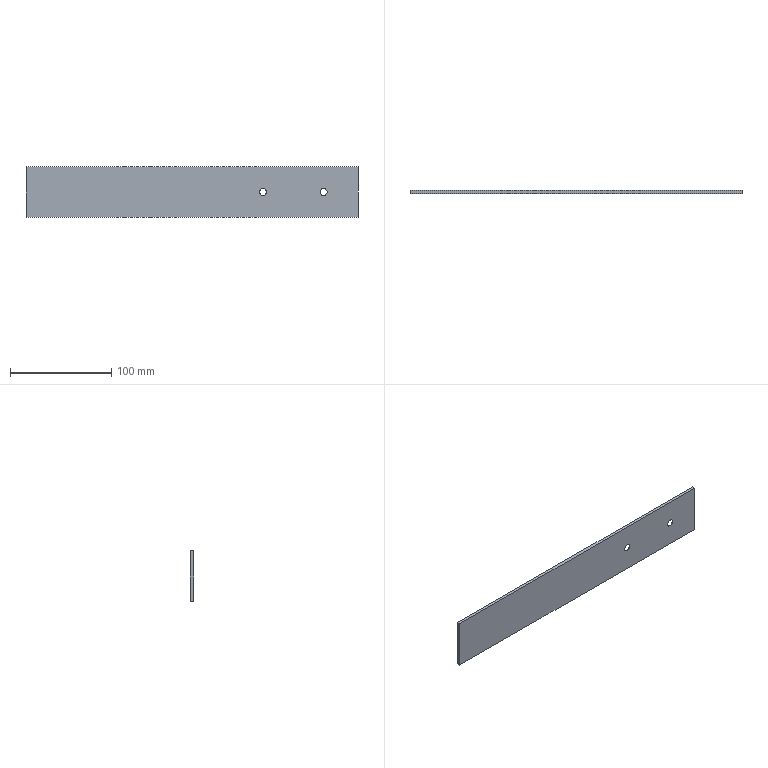Part | STEP file | Guard plate | 1 solid | 10 faces | box 328 x 3 x 50 mm | volume 48733 mm3 | plane 6 | cone 4
STEP:
#1=CARTESIAN_POINT('',(30.,-3.,3.4));
#2=VERTEX_POINT('',#1);
#3=CARTESIAN_POINT('',(30.,-3.,-3.4));
#4=VERTEX_POINT('',#3);
#5=CARTESIAN_POINT('',(30.,-3.,0.));
#6=DIRECTION('',(0.,-1.,0.));
#7=DIRECTION('',(0.,0.,1.));
#8=AXIS2_PLACEMENT_3D('',#5,#6,#7);
#9=CIRCLE('',#8,3.4);
#10=EDGE_CURVE('',#2,#4,#9,.T.);
#11=ORIENTED_EDGE('',*,*,#10,.T.);
#12=CARTESIAN_POINT('',(30.,0.,-6.4));
#13=VERTEX_POINT('',#12);
#14=CARTESIAN_POINT('',(30.,0.,-6.4));
#15=DIRECTION('',(0.,0.7071,-0.7071));
#16=VECTOR('',#15,1000.);
#17=LINE('',#14,#16);
#18=EDGE_CURVE('',#4,#13,#17,.T.);
#19=ORIENTED_EDGE('',*,*,#18,.T.);
#20=CARTESIAN_POINT('',(30.,0.,6.4));
#21=VERTEX_POINT('',#20);
#22=CARTESIAN_POINT('',(30.,0.,0.));
#23=DIRECTION('',(0.,-1.,0.));
#24=DIRECTION('',(0.,0.,1.));
#25=AXIS2_PLACEMENT_3D('',#22,#23,#24);
#26=CIRCLE('',#25,6.4);
#27=EDGE_CURVE('',#21,#13,#26,.T.);
#28=ORIENTED_EDGE('',*,*,#27,.F.);
#29=CARTESIAN_POINT('',(30.,0.,6.4));
#30=DIRECTION('',(0.,0.7071,0.7071));
#31=VECTOR('',#30,1000.);
#32=LINE('',#29,#31);
#33=EDGE_CURVE('',#2,#21,#32,.T.);
#34=ORIENTED_EDGE('',*,*,#33,.F.);
#35=EDGE_LOOP('',(#11,#19,#28,#34));
#36=FACE_OUTER_BOUND('',#35,.T.);
#37=CARTESIAN_POINT('',(30.,0.,0.));
#38=DIRECTION('',(0.,1.,0.));
#39=DIRECTION('',(0.,0.,1.));
#40=AXIS2_PLACEMENT_3D('',#37,#38,#39);
#41=CONICAL_SURFACE('',#40,6.4,0.7854);
#42=ADVANCED_FACE('',(#36),#41,.F.);
#43=CARTESIAN_POINT('',(-30.,-3.,3.4));
#44=VERTEX_POINT('',#43);
#45=CARTESIAN_POINT('',(-30.,-3.,-3.4));
#46=VERTEX_POINT('',#45);
#47=CARTESIAN_POINT('',(-30.,-3.,0.));
#48=DIRECTION('',(0.,-1.,0.));
#49=DIRECTION('',(0.,0.,1.));
#50=AXIS2_PLACEMENT_3D('',#47,#48,#49);
#51=CIRCLE('',#50,3.4);
#52=EDGE_CURVE('',#44,#46,#51,.T.);
#53=ORIENTED_EDGE('',*,*,#52,.T.);
#54=CARTESIAN_POINT('',(-30.,0.,-6.4));
#55=VERTEX_POINT('',#54);
#56=CARTESIAN_POINT('',(-30.,0.,-6.4));
#57=DIRECTION('',(0.,0.7071,-0.7071));
#58=VECTOR('',#57,1000.);
#59=LINE('',#56,#58);
#60=EDGE_CURVE('',#46,#55,#59,.T.);
#61=ORIENTED_EDGE('',*,*,#60,.T.);
#62=CARTESIAN_POINT('',(-30.,0.,6.4));
#63=VERTEX_POINT('',#62);
#64=CARTESIAN_POINT('',(-30.,0.,0.));
#65=DIRECTION('',(0.,-1.,0.));
#66=DIRECTION('',(0.,0.,1.));
#67=AXIS2_PLACEMENT_3D('',#64,#65,#66);
#68=CIRCLE('',#67,6.4);
#69=EDGE_CURVE('',#63,#55,#68,.T.);
#70=ORIENTED_EDGE('',*,*,#69,.F.);
#71=CARTESIAN_POINT('',(-30.,0.,6.4));
#72=DIRECTION('',(0.,0.7071,0.7071));
#73=VECTOR('',#72,1000.);
#74=LINE('',#71,#73);
#75=EDGE_CURVE('',#44,#63,#74,.T.);
#76=ORIENTED_EDGE('',*,*,#75,.F.);
#77=EDGE_LOOP('',(#53,#61,#70,#76));
#78=FACE_OUTER_BOUND('',#77,.T.);
#79=CARTESIAN_POINT('',(-30.,0.,0.));
#80=DIRECTION('',(0.,1.,0.));
#81=DIRECTION('',(0.,0.,1.));
#82=AXIS2_PLACEMENT_3D('',#79,#80,#81);
#83=CONICAL_SURFACE('',#82,6.4,0.7854);
#84=ADVANCED_FACE('',(#78),#83,.F.);
#85=CARTESIAN_POINT('',(-264.,-3.,25.));
#86=VERTEX_POINT('',#85);
#87=CARTESIAN_POINT('',(64.,-3.,25.));
#88=VERTEX_POINT('',#87);
#89=CARTESIAN_POINT('',(0.,-3.,25.));
#90=DIRECTION('',(1.,0.,0.));
#91=VECTOR('',#90,1000.);
#92=LINE('',#89,#91);
#93=EDGE_CURVE('',#86,#88,#92,.T.);
#94=ORIENTED_EDGE('',*,*,#93,.F.);
#95=CARTESIAN_POINT('',(-264.,-3.,-25.));
#96=VERTEX_POINT('',#95);
#97=CARTESIAN_POINT('',(-264.,-3.,-25.));
#98=DIRECTION('',(0.,0.,1.));
#99=VECTOR('',#98,1000.);
#100=LINE('',#97,#99);
#101=EDGE_CURVE('',#96,#86,#100,.T.);
#102=ORIENTED_EDGE('',*,*,#101,.F.);
#103=CARTESIAN_POINT('',(64.,-3.,-25.));
#104=VERTEX_POINT('',#103);
#105=CARTESIAN_POINT('',(0.,-3.,-25.));
#106=DIRECTION('',(-1.,0.,0.));
#107=VECTOR('',#106,1000.);
#108=LINE('',#105,#107);
#109=EDGE_CURVE('',#104,#96,#108,.T.);
#110=ORIENTED_EDGE('',*,*,#109,.F.);
#111=CARTESIAN_POINT('',(64.,-3.,0.));
#112=DIRECTION('',(0.,0.,-1.));
#113=VECTOR('',#112,1000.);
#114=LINE('',#111,#113);
#115=EDGE_CURVE('',#88,#104,#114,.T.);
#116=ORIENTED_EDGE('',*,*,#115,.F.);
#117=EDGE_LOOP('',(#94,#102,#110,#116));
#118=FACE_OUTER_BOUND('',#117,.T.);
#119=ORIENTED_EDGE('',*,*,#10,.F.);
#120=CARTESIAN_POINT('',(30.,-3.,0.));
#121=DIRECTION('',(0.,-1.,0.));
#122=DIRECTION('',(0.,0.,1.));
#123=AXIS2_PLACEMENT_3D('',#120,#121,#122);
#124=CIRCLE('',#123,3.4);
#125=EDGE_CURVE('',#4,#2,#124,.T.);
#126=ORIENTED_EDGE('',*,*,#125,.F.);
#127=EDGE_LOOP('',(#119,#126));
#128=FACE_BOUND('',#127,.T.);
#129=ORIENTED_EDGE('',*,*,#52,.F.);
#130=CARTESIAN_POINT('',(-30.,-3.,0.));
#131=DIRECTION('',(0.,-1.,0.));
#132=DIRECTION('',(0.,0.,1.));
#133=AXIS2_PLACEMENT_3D('',#130,#131,#132);
#134=CIRCLE('',#133,3.4);
#135=EDGE_CURVE('',#46,#44,#134,.T.);
#136=ORIENTED_EDGE('',*,*,#135,.F.);
#137=EDGE_LOOP('',(#129,#136));
#138=FACE_BOUND('',#137,.T.);
#139=CARTESIAN_POINT('',(0.,-3.,0.));
#140=DIRECTION('',(0.,1.,0.));
#141=DIRECTION('',(0.,0.,1.));
#142=AXIS2_PLACEMENT_3D('',#139,#140,#141);
#143=PLANE('',#142);
#144=ADVANCED_FACE('',(#118,#128,#138),#143,.F.);
#145=ORIENTED_EDGE('',*,*,#115,.T.);
#146=CARTESIAN_POINT('',(64.,0.,-25.));
#147=VERTEX_POINT('',#146);
#148=CARTESIAN_POINT('',(64.,-3.,-25.));
#149=DIRECTION('',(0.,1.,0.));
#150=VECTOR('',#149,1000.);
#151=LINE('',#148,#150);
#152=EDGE_CURVE('',#104,#147,#151,.T.);
#153=ORIENTED_EDGE('',*,*,#152,.T.);
#154=CARTESIAN_POINT('',(64.,0.,25.));
#155=VERTEX_POINT('',#154);
#156=CARTESIAN_POINT('',(64.,0.,-25.));
#157=DIRECTION('',(0.,0.,1.));
#158=VECTOR('',#157,1000.);
#159=LINE('',#156,#158);
#160=EDGE_CURVE('',#147,#155,#159,.T.);
#161=ORIENTED_EDGE('',*,*,#160,.T.);
#162=CARTESIAN_POINT('',(64.,-3.,25.));
#163=DIRECTION('',(0.,-1.,0.));
#164=VECTOR('',#163,1000.);
#165=LINE('',#162,#164);
#166=EDGE_CURVE('',#155,#88,#165,.T.);
#167=ORIENTED_EDGE('',*,*,#166,.T.);
#168=EDGE_LOOP('',(#145,#153,#161,#167));
#169=FACE_OUTER_BOUND('',#168,.T.);
#170=CARTESIAN_POINT('',(64.,-3.,-25.));
#171=DIRECTION('',(1.,0.,0.));
#172=DIRECTION('',(0.,0.,-1.));
#173=AXIS2_PLACEMENT_3D('',#170,#171,#172);
#174=PLANE('',#173);
#175=ADVANCED_FACE('',(#169),#174,.T.);
#176=ORIENTED_EDGE('',*,*,#93,.T.);
#177=ORIENTED_EDGE('',*,*,#166,.F.);
#178=CARTESIAN_POINT('',(-264.,0.,25.));
#179=VERTEX_POINT('',#178);
#180=CARTESIAN_POINT('',(-64.,0.,25.));
#181=DIRECTION('',(-1.,0.,0.));
#182=VECTOR('',#181,1000.);
#183=LINE('',#180,#182);
#184=EDGE_CURVE('',#155,#179,#183,.T.);
#185=ORIENTED_EDGE('',*,*,#184,.T.);
#186=CARTESIAN_POINT('',(-264.,-3.,25.));
#187=DIRECTION('',(0.,1.,0.));
#188=VECTOR('',#187,1000.);
#189=LINE('',#186,#188);
#190=EDGE_CURVE('',#86,#179,#189,.T.);
#191=ORIENTED_EDGE('',*,*,#190,.F.);
#192=EDGE_LOOP('',(#176,#177,#185,#191));
#193=FACE_OUTER_BOUND('',#192,.T.);
#194=CARTESIAN_POINT('',(-64.,-3.,25.));
#195=DIRECTION('',(0.,0.,1.));
#196=DIRECTION('',(1.,0.,0.));
#197=AXIS2_PLACEMENT_3D('',#194,#195,#196);
#198=PLANE('',#197);
#199=ADVANCED_FACE('',(#193),#198,.T.);
#200=ORIENTED_EDGE('',*,*,#109,.T.);
#201=CARTESIAN_POINT('',(-264.,0.,-25.));
#202=VERTEX_POINT('',#201);
#203=CARTESIAN_POINT('',(-264.,0.,-25.));
#204=DIRECTION('',(0.,-1.,0.));
#205=VECTOR('',#204,1000.);
#206=LINE('',#203,#205);
#207=EDGE_CURVE('',#202,#96,#206,.T.);
#208=ORIENTED_EDGE('',*,*,#207,.F.);
#209=CARTESIAN_POINT('',(-64.,0.,-25.));
#210=DIRECTION('',(1.,0.,0.));
#211=VECTOR('',#210,1000.);
#212=LINE('',#209,#211);
#213=EDGE_CURVE('',#202,#147,#212,.T.);
#214=ORIENTED_EDGE('',*,*,#213,.T.);
#215=ORIENTED_EDGE('',*,*,#152,.F.);
#216=EDGE_LOOP('',(#200,#208,#214,#215));
#217=FACE_OUTER_BOUND('',#216,.T.);
#218=CARTESIAN_POINT('',(-64.,-3.,-25.));
#219=DIRECTION('',(0.,0.,-1.));
#220=DIRECTION('',(-1.,0.,0.));
#221=AXIS2_PLACEMENT_3D('',#218,#219,#220);
#222=PLANE('',#221);
#223=ADVANCED_FACE('',(#217),#222,.T.);
#224=ORIENTED_EDGE('',*,*,#18,.F.);
#225=ORIENTED_EDGE('',*,*,#125,.T.);
#226=ORIENTED_EDGE('',*,*,#33,.T.);
#227=CARTESIAN_POINT('',(30.,0.,0.));
#228=DIRECTION('',(0.,-1.,0.));
#229=DIRECTION('',(0.,0.,1.));
#230=AXIS2_PLACEMENT_3D('',#227,#228,#229);
#231=CIRCLE('',#230,6.4);
#232=EDGE_CURVE('',#13,#21,#231,.T.);
#233=ORIENTED_EDGE('',*,*,#232,.F.);
#234=EDGE_LOOP('',(#224,#225,#226,#233));
#235=FACE_OUTER_BOUND('',#234,.T.);
#236=CARTESIAN_POINT('',(30.,0.,0.));
#237=DIRECTION('',(0.,1.,0.));
#238=DIRECTION('',(0.,0.,1.));
#239=AXIS2_PLACEMENT_3D('',#236,#237,#238);
#240=CONICAL_SURFACE('',#239,6.4,0.7854);
#241=ADVANCED_FACE('',(#235),#240,.F.);
#242=ORIENTED_EDGE('',*,*,#60,.F.);
#243=ORIENTED_EDGE('',*,*,#135,.T.);
#244=ORIENTED_EDGE('',*,*,#75,.T.);
#245=CARTESIAN_POINT('',(-30.,0.,0.));
#246=DIRECTION('',(0.,-1.,0.));
#247=DIRECTION('',(0.,0.,1.));
#248=AXIS2_PLACEMENT_3D('',#245,#246,#247);
#249=CIRCLE('',#248,6.4);
#250=EDGE_CURVE('',#55,#63,#249,.T.);
#251=ORIENTED_EDGE('',*,*,#250,.F.);
#252=EDGE_LOOP('',(#242,#243,#244,#251));
#253=FACE_OUTER_BOUND('',#252,.T.);
#254=CARTESIAN_POINT('',(-30.,0.,0.));
#255=DIRECTION('',(0.,1.,0.));
#256=DIRECTION('',(0.,0.,1.));
#257=AXIS2_PLACEMENT_3D('',#254,#255,#256);
#258=CONICAL_SURFACE('',#257,6.4,0.7854);
#259=ADVANCED_FACE('',(#253),#258,.F.);
#260=ORIENTED_EDGE('',*,*,#213,.F.);
#261=CARTESIAN_POINT('',(-264.,0.,25.));
#262=DIRECTION('',(0.,0.,-1.));
#263=VECTOR('',#262,1000.);
#264=LINE('',#261,#263);
#265=EDGE_CURVE('',#179,#202,#264,.T.);
#266=ORIENTED_EDGE('',*,*,#265,.F.);
#267=ORIENTED_EDGE('',*,*,#184,.F.);
#268=ORIENTED_EDGE('',*,*,#160,.F.);
#269=EDGE_LOOP('',(#260,#266,#267,#268));
#270=FACE_OUTER_BOUND('',#269,.T.);
#271=ORIENTED_EDGE('',*,*,#27,.T.);
#272=ORIENTED_EDGE('',*,*,#232,.T.);
#273=EDGE_LOOP('',(#271,#272));
#274=FACE_BOUND('',#273,.T.);
#275=ORIENTED_EDGE('',*,*,#69,.T.);
#276=ORIENTED_EDGE('',*,*,#250,.T.);
#277=EDGE_LOOP('',(#275,#276));
#278=FACE_BOUND('',#277,.T.);
#279=CARTESIAN_POINT('',(0.,0.,0.));
#280=DIRECTION('',(0.,1.,0.));
#281=DIRECTION('',(0.,0.,1.));
#282=AXIS2_PLACEMENT_3D('',#279,#280,#281);
#283=PLANE('',#282);
#284=ADVANCED_FACE('',(#270,#274,#278),#283,.T.);
#285=ORIENTED_EDGE('',*,*,#207,.T.);
#286=ORIENTED_EDGE('',*,*,#101,.T.);
#287=ORIENTED_EDGE('',*,*,#190,.T.);
#288=ORIENTED_EDGE('',*,*,#265,.T.);
#289=EDGE_LOOP('',(#285,#286,#287,#288));
#290=FACE_OUTER_BOUND('',#289,.T.);
#291=CARTESIAN_POINT('',(-264.,0.,0.));
#292=DIRECTION('',(-1.,0.,0.));
#293=DIRECTION('',(0.,0.,1.));
#294=AXIS2_PLACEMENT_3D('',#291,#292,#293);
#295=PLANE('',#294);
#296=ADVANCED_FACE('',(#290),#295,.T.);
#297=CLOSED_SHELL('',(#42,#84,#144,#175,#199,#223,#241,#259,#284,#296));
#298=MANIFOLD_SOLID_BREP('',#297);
#299=CARTESIAN_POINT('',(0.,0.,0.));
#300=DIRECTION('',(0.,0.,1.));
#301=DIRECTION('',(1.,0.,0.));
#302=AXIS2_PLACEMENT_3D('',#299,#300,#301);
#303=(LENGTH_UNIT()NAMED_UNIT(*)SI_UNIT(.MILLI.,.METRE.));
#304=UNCERTAINTY_MEASURE_WITH_UNIT(LENGTH_MEASURE(0.00001),#303,'','');
#305=(NAMED_UNIT(*)PLANE_ANGLE_UNIT()SI_UNIT($,.RADIAN.));
#306=(NAMED_UNIT(*)SI_UNIT($,.STERADIAN.)SOLID_ANGLE_UNIT());
#307=(GEOMETRIC_REPRESENTATION_CONTEXT(3)GLOBAL_UNCERTAINTY_ASSIGNED_CONTEXT((#304))GLOBAL_UNIT_ASSIGNED_CONTEXT((#303,#305,#306))REPRESENTATION_CONTEXT('',''));
#308=ADVANCED_BREP_SHAPE_REPRESENTATION('',(#298,#302),#307);